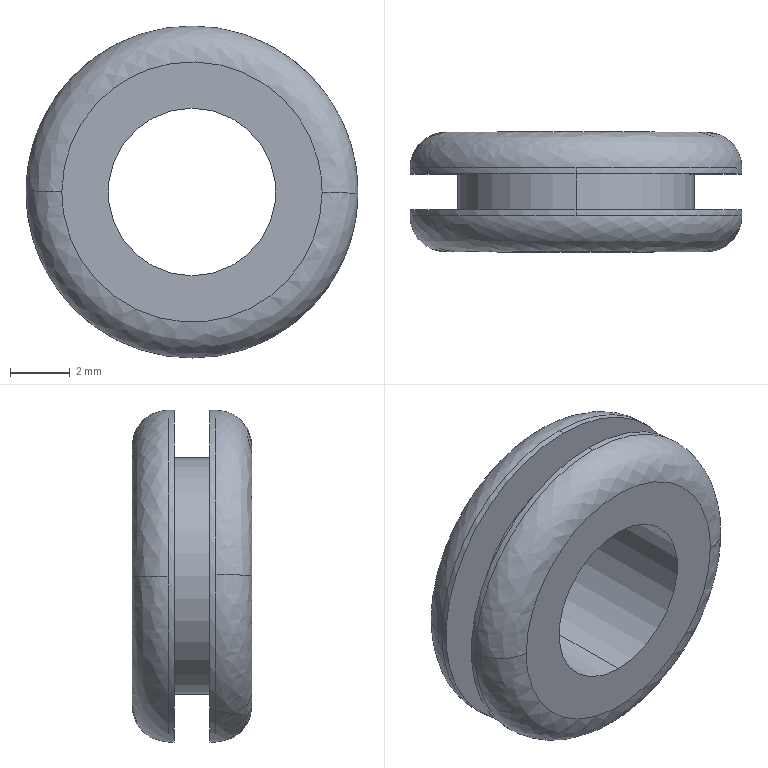Part | SolidWorks | features BaseBody 1 | 1 solid | 16 faces | box 11.1 x 4 x 11.1 mm | volume 210.744 mm3 | cylinder 8 | plane 4 | spline 4 | commonest cylinder face diameters 11.1 x4 5.6 x2 7.9 x2
STEP:
#1=CARTESIAN_POINT('',(0.,1.4,3.95));
#2=VERTEX_POINT('',#1);
#3=CARTESIAN_POINT('',(0.,1.4,-3.95));
#4=VERTEX_POINT('',#3);
#5=CARTESIAN_POINT('',(0.,1.4,0.));
#6=DIRECTION('',(0.,-1.,0.));
#7=DIRECTION('',(0.,0.,1.));
#8=AXIS2_PLACEMENT_3D('',#5,#6,#7);
#9=CIRCLE('',#8,3.95);
#10=EDGE_CURVE('',#2,#4,#9,.T.);
#11=ORIENTED_EDGE('',*,*,#10,.T.);
#12=CARTESIAN_POINT('',(0.,1.4,0.));
#13=DIRECTION('',(0.,-1.,0.));
#14=DIRECTION('',(0.,0.,1.));
#15=AXIS2_PLACEMENT_3D('',#12,#13,#14);
#16=CIRCLE('',#15,3.95);
#17=EDGE_CURVE('',#4,#2,#16,.T.);
#18=ORIENTED_EDGE('',*,*,#17,.T.);
#19=EDGE_LOOP('',(#11,#18));
#20=FACE_BOUND('',#19,.T.);
#21=CARTESIAN_POINT('',(0.,1.4,5.55));
#22=VERTEX_POINT('',#21);
#23=CARTESIAN_POINT('',(0.,1.4,-5.55));
#24=VERTEX_POINT('',#23);
#25=CARTESIAN_POINT('',(0.,1.4,0.));
#26=DIRECTION('',(0.,1.,0.));
#27=DIRECTION('',(0.,0.,1.));
#28=AXIS2_PLACEMENT_3D('',#25,#26,#27);
#29=CIRCLE('',#28,5.55);
#30=EDGE_CURVE('',#22,#24,#29,.T.);
#31=ORIENTED_EDGE('',*,*,#30,.T.);
#32=CARTESIAN_POINT('',(0.,1.4,0.));
#33=DIRECTION('',(0.,1.,0.));
#34=DIRECTION('',(0.,0.,1.));
#35=AXIS2_PLACEMENT_3D('',#32,#33,#34);
#36=CIRCLE('',#35,5.55);
#37=EDGE_CURVE('',#24,#22,#36,.T.);
#38=ORIENTED_EDGE('',*,*,#37,.T.);
#39=EDGE_LOOP('',(#31,#38));
#40=FACE_OUTER_BOUND('',#39,.T.);
#41=CARTESIAN_POINT('',(0.,1.4,0.));
#42=DIRECTION('',(0.,1.,0.));
#43=DIRECTION('',(1.,0.,0.));
#44=AXIS2_PLACEMENT_3D('',#41,#42,#43);
#45=PLANE('',#44);
#46=ADVANCED_FACE('',(#20,#40),#45,.T.);
#47=CARTESIAN_POINT('',(0.,2.6,-3.95));
#48=VERTEX_POINT('',#47);
#49=CARTESIAN_POINT('',(0.,1.4,-3.95));
#50=DIRECTION('',(0.,1.,0.));
#51=VECTOR('',#50,1000.);
#52=LINE('',#49,#51);
#53=EDGE_CURVE('',#4,#48,#52,.T.);
#54=ORIENTED_EDGE('',*,*,#53,.F.);
#55=ORIENTED_EDGE('',*,*,#10,.F.);
#56=CARTESIAN_POINT('',(0.,2.6,3.95));
#57=VERTEX_POINT('',#56);
#58=CARTESIAN_POINT('',(0.,1.4,3.95));
#59=DIRECTION('',(0.,1.,0.));
#60=VECTOR('',#59,1000.);
#61=LINE('',#58,#60);
#62=EDGE_CURVE('',#2,#57,#61,.T.);
#63=ORIENTED_EDGE('',*,*,#62,.T.);
#64=CARTESIAN_POINT('',(0.,2.6,0.));
#65=DIRECTION('',(0.,-1.,0.));
#66=DIRECTION('',(0.,0.,1.));
#67=AXIS2_PLACEMENT_3D('',#64,#65,#66);
#68=CIRCLE('',#67,3.95);
#69=EDGE_CURVE('',#57,#48,#68,.T.);
#70=ORIENTED_EDGE('',*,*,#69,.T.);
#71=EDGE_LOOP('',(#54,#55,#63,#70));
#72=FACE_OUTER_BOUND('',#71,.T.);
#73=CARTESIAN_POINT('',(0.,1.4,0.));
#74=DIRECTION('',(0.,1.,0.));
#75=DIRECTION('',(0.,0.,1.));
#76=AXIS2_PLACEMENT_3D('',#73,#74,#75);
#77=CYLINDRICAL_SURFACE('',#76,3.95);
#78=ADVANCED_FACE('',(#72),#77,.T.);
#79=CARTESIAN_POINT('',(0.,1.2,-5.55));
#80=VERTEX_POINT('',#79);
#81=CARTESIAN_POINT('',(0.,0.,-5.55));
#82=DIRECTION('',(0.,1.,0.));
#83=VECTOR('',#82,1000.);
#84=LINE('',#81,#83);
#85=EDGE_CURVE('',#80,#24,#84,.T.);
#86=ORIENTED_EDGE('',*,*,#85,.F.);
#87=CARTESIAN_POINT('',(-5.55,1.2,0.0354));
#88=VERTEX_POINT('',#87);
#89=CARTESIAN_POINT('',(0.,1.2,0.));
#90=DIRECTION('',(0.,1.,0.));
#91=DIRECTION('',(0.,0.,1.));
#92=AXIS2_PLACEMENT_3D('',#89,#90,#91);
#93=CIRCLE('',#92,5.55);
#94=EDGE_CURVE('',#80,#88,#93,.T.);
#95=ORIENTED_EDGE('',*,*,#94,.T.);
#96=CARTESIAN_POINT('',(0.,1.2,5.55));
#97=VERTEX_POINT('',#96);
#98=CARTESIAN_POINT('',(0.,1.2,0.));
#99=DIRECTION('',(0.,1.,0.));
#100=DIRECTION('',(0.,0.,1.));
#101=AXIS2_PLACEMENT_3D('',#98,#99,#100);
#102=CIRCLE('',#101,5.55);
#103=EDGE_CURVE('',#88,#97,#102,.T.);
#104=ORIENTED_EDGE('',*,*,#103,.T.);
#105=CARTESIAN_POINT('',(0.,0.,5.55));
#106=DIRECTION('',(0.,1.,0.));
#107=VECTOR('',#106,1000.);
#108=LINE('',#105,#107);
#109=EDGE_CURVE('',#97,#22,#108,.T.);
#110=ORIENTED_EDGE('',*,*,#109,.T.);
#111=ORIENTED_EDGE('',*,*,#37,.F.);
#112=EDGE_LOOP('',(#86,#95,#104,#110,#111));
#113=FACE_OUTER_BOUND('',#112,.T.);
#114=CARTESIAN_POINT('',(0.,0.,0.));
#115=DIRECTION('',(0.,1.,0.));
#116=DIRECTION('',(0.,0.,1.));
#117=AXIS2_PLACEMENT_3D('',#114,#115,#116);
#118=CYLINDRICAL_SURFACE('',#117,5.55);
#119=ADVANCED_FACE('',(#113),#118,.T.);
#120=ORIENTED_EDGE('',*,*,#69,.F.);
#121=CARTESIAN_POINT('',(0.,2.6,0.));
#122=DIRECTION('',(0.,-1.,0.));
#123=DIRECTION('',(0.,0.,1.));
#124=AXIS2_PLACEMENT_3D('',#121,#122,#123);
#125=CIRCLE('',#124,3.95);
#126=EDGE_CURVE('',#48,#57,#125,.T.);
#127=ORIENTED_EDGE('',*,*,#126,.F.);
#128=EDGE_LOOP('',(#120,#127));
#129=FACE_BOUND('',#128,.T.);
#130=CARTESIAN_POINT('',(0.,2.6,5.55));
#131=VERTEX_POINT('',#130);
#132=CARTESIAN_POINT('',(0.,2.6,-5.55));
#133=VERTEX_POINT('',#132);
#134=CARTESIAN_POINT('',(0.,2.6,0.));
#135=DIRECTION('',(0.,1.,0.));
#136=DIRECTION('',(0.,0.,1.));
#137=AXIS2_PLACEMENT_3D('',#134,#135,#136);
#138=CIRCLE('',#137,5.55);
#139=EDGE_CURVE('',#131,#133,#138,.T.);
#140=ORIENTED_EDGE('',*,*,#139,.F.);
#141=CARTESIAN_POINT('',(0.,2.6,0.));
#142=DIRECTION('',(0.,1.,0.));
#143=DIRECTION('',(0.,0.,1.));
#144=AXIS2_PLACEMENT_3D('',#141,#142,#143);
#145=CIRCLE('',#144,5.55);
#146=EDGE_CURVE('',#133,#131,#145,.T.);
#147=ORIENTED_EDGE('',*,*,#146,.F.);
#148=EDGE_LOOP('',(#140,#147));
#149=FACE_OUTER_BOUND('',#148,.T.);
#150=CARTESIAN_POINT('',(0.,2.6,0.));
#151=DIRECTION('',(0.,1.,0.));
#152=DIRECTION('',(1.,0.,0.));
#153=AXIS2_PLACEMENT_3D('',#150,#151,#152);
#154=PLANE('',#153);
#155=ADVANCED_FACE('',(#129,#149),#154,.F.);
#156=CARTESIAN_POINT('',(5.55,1.2,-0.0354));
#157=VERTEX_POINT('',#156);
#158=CARTESIAN_POINT('',(4.35,0.,-0.02774));
#159=VERTEX_POINT('',#158);
#160=CARTESIAN_POINT('',(4.35,1.2,-0.02774));
#161=DIRECTION('',(-0.006378,0.,-1.));
#162=DIRECTION('',(1.,0.,-0.006378));
#163=AXIS2_PLACEMENT_3D('',#160,#161,#162);
#164=CIRCLE('',#163,1.2);
#165=EDGE_CURVE('',#157,#159,#164,.T.);
#166=ORIENTED_EDGE('',*,*,#165,.F.);
#167=CARTESIAN_POINT('',(0.,1.2,0.));
#168=DIRECTION('',(0.,1.,0.));
#169=DIRECTION('',(0.,0.,1.));
#170=AXIS2_PLACEMENT_3D('',#167,#168,#169);
#171=CIRCLE('',#170,5.55);
#172=EDGE_CURVE('',#97,#157,#171,.T.);
#173=ORIENTED_EDGE('',*,*,#172,.F.);
#174=ORIENTED_EDGE('',*,*,#103,.F.);
#175=CARTESIAN_POINT('',(-4.35,0.,0.02774));
#176=VERTEX_POINT('',#175);
#177=CARTESIAN_POINT('',(-4.35,1.2,0.02774));
#178=DIRECTION('',(0.006378,0.,1.));
#179=DIRECTION('',(-1.,0.,0.006378));
#180=AXIS2_PLACEMENT_3D('',#177,#178,#179);
#181=CIRCLE('',#180,1.2);
#182=EDGE_CURVE('',#88,#176,#181,.T.);
#183=ORIENTED_EDGE('',*,*,#182,.T.);
#184=CARTESIAN_POINT('',(4.35,0.,0.));
#185=VERTEX_POINT('',#184);
#186=CARTESIAN_POINT('',(-4.35,0.,0.02774));
#187=CARTESIAN_POINT('',(-4.347,0.,0.4058));
#188=CARTESIAN_POINT('',(-4.295,0.00000001,0.833));
#189=CARTESIAN_POINT('',(-4.016,0.000000026,1.737));
#190=CARTESIAN_POINT('',(-3.787,0.000000032,2.214));
#191=CARTESIAN_POINT('',(-3.091,0.000000032,3.113));
#192=CARTESIAN_POINT('',(-2.622,0.000000026,3.533));
#193=CARTESIAN_POINT('',(-1.743,0.000000014,3.999));
#194=CARTESIAN_POINT('',(-1.421,0.00000001,4.126));
#195=CARTESIAN_POINT('',(-0.9047,0.000000004,4.258));
#196=CARTESIAN_POINT('',(-0.7269,0.000000003,4.293));
#197=CARTESIAN_POINT('',(-0.4535,0.000000001,4.327));
#198=CARTESIAN_POINT('',(-0.3613,0.000000001,4.336));
#199=CARTESIAN_POINT('',(-0.2216,0.,4.345));
#200=CARTESIAN_POINT('',(-0.1514,0.,4.348));
#201=CARTESIAN_POINT('',(-0.06892,0.,4.35));
#202=CARTESIAN_POINT('',(-0.02757,0.,4.35));
#203=CARTESIAN_POINT('',(-0.009816,0.,4.35));
#204=CARTESIAN_POINT('',(0.002023,0.,4.35));
#205=CARTESIAN_POINT('',(0.009432,0.,4.35));
#206=CARTESIAN_POINT('',(0.5821,0.,4.348));
#207=CARTESIAN_POINT('',(1.15,0.000000006,4.234));
#208=CARTESIAN_POINT('',(2.199,0.000000015,3.796));
#209=CARTESIAN_POINT('',(2.68,0.000000018,3.474));
#210=CARTESIAN_POINT('',(3.482,0.000000018,2.669));
#211=CARTESIAN_POINT('',(3.803,0.000000015,2.187));
#212=CARTESIAN_POINT('',(4.237,0.000000006,1.136));
#213=CARTESIAN_POINT('',(4.35,0.,0.5683));
#214=CARTESIAN_POINT('',(4.35,0.,0.));
#215=B_SPLINE_CURVE_WITH_KNOTS('',3,(#186,#187,#188,#189,#190,#191,#192,#193,#194,#195,#196,#197,#198,#199,#200,#201,#202,#203,#204,#205,#206,#207,#208,#209,#210,#211,#212,#213,#214),.UNSPECIFIED.,.F.,.F.,(4,2,2,2,2,2,2,1,1,1,2,2,2,2,2,4),(0.,0.125,0.25,0.375,0.4375,0.4688,0.4844,0.4922,0.4961,0.498,0.499,0.5,0.625,0.75,0.875,1.),.UNSPECIFIED.);
#216=EDGE_CURVE('',#176,#185,#215,.T.);
#217=ORIENTED_EDGE('',*,*,#216,.T.);
#218=CARTESIAN_POINT('',(4.35,0.,-0.02774));
#219=DIRECTION('',(-0.003189,0.,-1.));
#220=VECTOR('',#219,1000.);
#221=LINE('',#218,#220);
#222=EDGE_CURVE('',#185,#159,#221,.T.);
#223=ORIENTED_EDGE('',*,*,#222,.T.);
#224=EDGE_LOOP('',(#166,#173,#174,#183,#217,#223));
#225=FACE_OUTER_BOUND('',#224,.T.);
#226=CARTESIAN_POINT('',(-5.55,1.2,0.0354));
#227=CARTESIAN_POINT('',(-5.479,1.2,11.135));
#228=CARTESIAN_POINT('',(5.621,1.2,11.064));
#229=CARTESIAN_POINT('',(5.55,1.2,-0.0354));
#230=CARTESIAN_POINT('',(-5.55,0.4917,0.0354));
#231=CARTESIAN_POINT('',(-5.479,0.4917,11.135));
#232=CARTESIAN_POINT('',(5.621,0.4917,11.064));
#233=CARTESIAN_POINT('',(5.55,0.4917,-0.0354));
#234=CARTESIAN_POINT('',(-5.047,-0.006784,0.03219));
#235=CARTESIAN_POINT('',(-4.982,-0.006784,10.125));
#236=CARTESIAN_POINT('',(5.111,-0.006784,10.061));
#237=CARTESIAN_POINT('',(5.047,-0.006784,-0.03219));
#238=CARTESIAN_POINT('',(-4.338,0.00005595,0.02767));
#239=CARTESIAN_POINT('',(-4.283,0.00005595,8.704));
#240=CARTESIAN_POINT('',(4.394,0.00005595,8.649));
#241=CARTESIAN_POINT('',(4.338,0.00005595,-0.02767));
#242=(BOUNDED_SURFACE()B_SPLINE_SURFACE(3,3,((#226,#227,#228,#229),(#230,#231,#232,#233),(#234,#235,#236,#237),(#238,#239,#240,#241)),.UNSPECIFIED.,.F.,.F.,.T.)B_SPLINE_SURFACE_WITH_KNOTS((4,4),(4,4),(0.,1.),(0.,1.),.UNSPECIFIED.)GEOMETRIC_REPRESENTATION_ITEM()RATIONAL_B_SPLINE_SURFACE(((1.,0.3333,0.3333,1.),(0.8025,0.2675,0.2675,0.8025),(0.8025,0.2675,0.2675,0.8025),(1.,0.3333,0.3333,1.)))REPRESENTATION_ITEM('')SURFACE());
#243=ADVANCED_FACE('',(#225),#242,.T.);
#244=CARTESIAN_POINT('',(0.,2.8,-5.55));
#245=VERTEX_POINT('',#244);
#246=CARTESIAN_POINT('',(0.,0.,-5.55));
#247=DIRECTION('',(0.,1.,0.));
#248=VECTOR('',#247,1000.);
#249=LINE('',#246,#248);
#250=EDGE_CURVE('',#133,#245,#249,.T.);
#251=ORIENTED_EDGE('',*,*,#250,.F.);
#252=ORIENTED_EDGE('',*,*,#146,.T.);
#253=CARTESIAN_POINT('',(0.,2.8,5.55));
#254=VERTEX_POINT('',#253);
#255=CARTESIAN_POINT('',(0.,0.,5.55));
#256=DIRECTION('',(0.,1.,0.));
#257=VECTOR('',#256,1000.);
#258=LINE('',#255,#257);
#259=EDGE_CURVE('',#131,#254,#258,.T.);
#260=ORIENTED_EDGE('',*,*,#259,.T.);
#261=CARTESIAN_POINT('',(-5.55,2.8,-0.02492));
#262=VERTEX_POINT('',#261);
#263=CARTESIAN_POINT('',(0.,2.8,0.));
#264=DIRECTION('',(0.,-1.,0.));
#265=DIRECTION('',(0.,0.,1.));
#266=AXIS2_PLACEMENT_3D('',#263,#264,#265);
#267=CIRCLE('',#266,5.55);
#268=EDGE_CURVE('',#254,#262,#267,.T.);
#269=ORIENTED_EDGE('',*,*,#268,.T.);
#270=CARTESIAN_POINT('',(0.,2.8,0.));
#271=DIRECTION('',(0.,-1.,0.));
#272=DIRECTION('',(0.,0.,1.));
#273=AXIS2_PLACEMENT_3D('',#270,#271,#272);
#274=CIRCLE('',#273,5.55);
#275=EDGE_CURVE('',#262,#245,#274,.T.);
#276=ORIENTED_EDGE('',*,*,#275,.T.);
#277=EDGE_LOOP('',(#251,#252,#260,#269,#276));
#278=FACE_OUTER_BOUND('',#277,.T.);
#279=CARTESIAN_POINT('',(0.,0.,0.));
#280=DIRECTION('',(0.,1.,0.));
#281=DIRECTION('',(0.,0.,1.));
#282=AXIS2_PLACEMENT_3D('',#279,#280,#281);
#283=CYLINDRICAL_SURFACE('',#282,5.55);
#284=ADVANCED_FACE('',(#278),#283,.T.);
#285=CARTESIAN_POINT('',(0.,0.,2.8));
#286=VERTEX_POINT('',#285);
#287=CARTESIAN_POINT('',(0.,0.,-2.8));
#288=VERTEX_POINT('',#287);
#289=CARTESIAN_POINT('',(0.,0.,0.));
#290=DIRECTION('',(0.,-1.,0.));
#291=DIRECTION('',(0.,0.,1.));
#292=AXIS2_PLACEMENT_3D('',#289,#290,#291);
#293=CIRCLE('',#292,2.8);
#294=EDGE_CURVE('',#286,#288,#293,.T.);
#295=ORIENTED_EDGE('',*,*,#294,.F.);
#296=CARTESIAN_POINT('',(0.,0.,0.));
#297=DIRECTION('',(0.,-1.,0.));
#298=DIRECTION('',(0.,0.,1.));
#299=AXIS2_PLACEMENT_3D('',#296,#297,#298);
#300=CIRCLE('',#299,2.8);
#301=EDGE_CURVE('',#288,#286,#300,.T.);
#302=ORIENTED_EDGE('',*,*,#301,.F.);
#303=EDGE_LOOP('',(#295,#302));
#304=FACE_BOUND('',#303,.T.);
#305=ORIENTED_EDGE('',*,*,#222,.F.);
#306=ORIENTED_EDGE('',*,*,#216,.F.);
#307=CARTESIAN_POINT('',(-4.35,0.,0.));
#308=VERTEX_POINT('',#307);
#309=CARTESIAN_POINT('',(-4.35,0.,0.02774));
#310=DIRECTION('',(0.003189,0.,1.));
#311=VECTOR('',#310,1000.);
#312=LINE('',#309,#311);
#313=EDGE_CURVE('',#308,#176,#312,.T.);
#314=ORIENTED_EDGE('',*,*,#313,.F.);
#315=CARTESIAN_POINT('',(4.35,0.,-0.02774));
#316=CARTESIAN_POINT('',(4.295,0.,-8.672));
#317=CARTESIAN_POINT('',(-4.35,0.,-8.645));
#318=CARTESIAN_POINT('',(-4.35,0.,0.));
#319=(BOUNDED_CURVE()B_SPLINE_CURVE(3,(#315,#316,#317,#318),.UNSPECIFIED.,.F.,.T.)B_SPLINE_CURVE_WITH_KNOTS((4,4),(0.,1.),.UNSPECIFIED.)CURVE()GEOMETRIC_REPRESENTATION_ITEM()RATIONAL_B_SPLINE_CURVE((1.,0.3355,0.3355,1.))REPRESENTATION_ITEM(''));
#320=EDGE_CURVE('',#159,#308,#319,.T.);
#321=ORIENTED_EDGE('',*,*,#320,.F.);
#322=EDGE_LOOP('',(#305,#306,#314,#321));
#323=FACE_OUTER_BOUND('',#322,.T.);
#324=CARTESIAN_POINT('',(0.,0.,0.));
#325=DIRECTION('',(0.,1.,0.));
#326=DIRECTION('',(1.,0.,0.));
#327=AXIS2_PLACEMENT_3D('',#324,#325,#326);
#328=PLANE('',#327);
#329=ADVANCED_FACE('',(#304,#323),#328,.F.);
#330=CARTESIAN_POINT('',(4.35,4.,0.01953));
#331=VERTEX_POINT('',#330);
#332=CARTESIAN_POINT('',(5.55,2.8,0.02492));
#333=VERTEX_POINT('',#332);
#334=CARTESIAN_POINT('',(4.35,2.8,0.01953));
#335=DIRECTION('',(0.00449,0.,-1.));
#336=DIRECTION('',(1.,0.,0.00449));
#337=AXIS2_PLACEMENT_3D('',#334,#335,#336);
#338=CIRCLE('',#337,1.2);
#339=EDGE_CURVE('',#331,#333,#338,.T.);
#340=ORIENTED_EDGE('',*,*,#339,.F.);
#341=CARTESIAN_POINT('',(-4.35,4.,0.));
#342=VERTEX_POINT('',#341);
#343=CARTESIAN_POINT('',(4.35,4.,0.01953));
#344=CARTESIAN_POINT('',(4.311,4.,8.681));
#345=CARTESIAN_POINT('',(-4.35,4.,8.661));
#346=CARTESIAN_POINT('',(-4.35,4.,0.));
#347=(BOUNDED_CURVE()B_SPLINE_CURVE(3,(#343,#344,#345,#346),.UNSPECIFIED.,.F.,.F.)B_SPLINE_CURVE_WITH_KNOTS((4,4),(0.,1.),.UNSPECIFIED.)CURVE()GEOMETRIC_REPRESENTATION_ITEM()RATIONAL_B_SPLINE_CURVE((1.,0.3348,0.3348,1.))REPRESENTATION_ITEM(''));
#348=EDGE_CURVE('',#331,#342,#347,.T.);
#349=ORIENTED_EDGE('',*,*,#348,.T.);
#350=CARTESIAN_POINT('',(-4.35,4.,-0.01953));
#351=VERTEX_POINT('',#350);
#352=CARTESIAN_POINT('',(-4.35,4.,-0.01953));
#353=DIRECTION('',(0.002245,0.,-1.));
#354=VECTOR('',#353,1000.);
#355=LINE('',#352,#354);
#356=EDGE_CURVE('',#342,#351,#355,.T.);
#357=ORIENTED_EDGE('',*,*,#356,.T.);
#358=CARTESIAN_POINT('',(-4.35,2.8,-0.01953));
#359=DIRECTION('',(-0.00449,0.,1.));
#360=DIRECTION('',(-1.,0.,-0.00449));
#361=AXIS2_PLACEMENT_3D('',#358,#359,#360);
#362=CIRCLE('',#361,1.2);
#363=EDGE_CURVE('',#351,#262,#362,.T.);
#364=ORIENTED_EDGE('',*,*,#363,.T.);
#365=ORIENTED_EDGE('',*,*,#268,.F.);
#366=CARTESIAN_POINT('',(0.,2.8,0.));
#367=DIRECTION('',(0.,-1.,0.));
#368=DIRECTION('',(0.,0.,1.));
#369=AXIS2_PLACEMENT_3D('',#366,#367,#368);
#370=CIRCLE('',#369,5.55);
#371=EDGE_CURVE('',#333,#254,#370,.T.);
#372=ORIENTED_EDGE('',*,*,#371,.F.);
#373=EDGE_LOOP('',(#340,#349,#357,#364,#365,#372));
#374=FACE_OUTER_BOUND('',#373,.T.);
#375=CARTESIAN_POINT('',(-4.339,4.,-0.01948));
#376=CARTESIAN_POINT('',(-4.35,4.,2.541));
#377=CARTESIAN_POINT('',(-2.539,4.,4.351));
#378=CARTESIAN_POINT('',(0.02141,4.,4.339));
#379=CARTESIAN_POINT('',(2.582,4.,4.326));
#380=CARTESIAN_POINT('',(4.375,4.,2.498));
#381=CARTESIAN_POINT('',(4.338,4.,-0.0623));
#382=CARTESIAN_POINT('',(-5.047,4.007,-0.02266));
#383=CARTESIAN_POINT('',(-5.06,4.007,2.956));
#384=CARTESIAN_POINT('',(-2.954,4.007,5.061));
#385=CARTESIAN_POINT('',(0.02491,4.007,5.047));
#386=CARTESIAN_POINT('',(3.003,4.007,5.032));
#387=CARTESIAN_POINT('',(5.089,4.007,2.906));
#388=CARTESIAN_POINT('',(5.046,4.007,-0.07247));
#389=CARTESIAN_POINT('',(-5.55,3.508,-0.02492));
#390=CARTESIAN_POINT('',(-5.565,3.508,3.251));
#391=CARTESIAN_POINT('',(-3.248,3.508,5.566));
#392=CARTESIAN_POINT('',(0.02739,3.508,5.55));
#393=CARTESIAN_POINT('',(3.303,3.508,5.534));
#394=CARTESIAN_POINT('',(5.596,3.508,3.195));
#395=CARTESIAN_POINT('',(5.549,3.508,-0.07969));
#396=CARTESIAN_POINT('',(-5.55,2.8,-0.02492));
#397=CARTESIAN_POINT('',(-5.565,2.8,3.251));
#398=CARTESIAN_POINT('',(-3.248,2.8,5.566));
#399=CARTESIAN_POINT('',(0.02739,2.8,5.55));
#400=CARTESIAN_POINT('',(3.303,2.8,5.534));
#401=CARTESIAN_POINT('',(5.596,2.8,3.195));
#402=CARTESIAN_POINT('',(5.549,2.8,-0.07969));
#403=(BOUNDED_SURFACE()B_SPLINE_SURFACE(3,3,((#375,#376,#377,#378,#379,#380,#381),(#382,#383,#384,#385,#386,#387,#388),(#389,#390,#391,#392,#393,#394,#395),(#396,#397,#398,#399,#400,#401,#402)),.UNSPECIFIED.,.F.,.F.,.T.)B_SPLINE_SURFACE_WITH_KNOTS((4,4),(4,3,4),(0.,1.),(0.,0.5,1.),.UNSPECIFIED.)GEOMETRIC_REPRESENTATION_ITEM()RATIONAL_B_SPLINE_SURFACE(((1.,0.8025,0.8025,1.,0.8025,0.8025,1.),(0.8025,0.644,0.644,0.8025,0.644,0.644,0.8025),(0.8025,0.644,0.644,0.8025,0.644,0.644,0.8025),(1.,0.8025,0.8025,1.,0.8025,0.8025,1.)))REPRESENTATION_ITEM('')SURFACE());
#404=ADVANCED_FACE('',(#374),#403,.T.);
#405=CARTESIAN_POINT('',(0.,4.,-2.8));
#406=VERTEX_POINT('',#405);
#407=CARTESIAN_POINT('',(0.,4.,-2.8));
#408=DIRECTION('',(0.,1.,0.));
#409=VECTOR('',#408,1000.);
#410=LINE('',#407,#409);
#411=EDGE_CURVE('',#288,#406,#410,.T.);
#412=ORIENTED_EDGE('',*,*,#411,.F.);
#413=ORIENTED_EDGE('',*,*,#301,.T.);
#414=CARTESIAN_POINT('',(0.,4.,2.8));
#415=VERTEX_POINT('',#414);
#416=CARTESIAN_POINT('',(0.,4.,2.8));
#417=DIRECTION('',(0.,1.,0.));
#418=VECTOR('',#417,1000.);
#419=LINE('',#416,#418);
#420=EDGE_CURVE('',#286,#415,#419,.T.);
#421=ORIENTED_EDGE('',*,*,#420,.T.);
#422=CARTESIAN_POINT('',(0.,4.,0.));
#423=DIRECTION('',(0.,-1.,0.));
#424=DIRECTION('',(0.,0.,1.));
#425=AXIS2_PLACEMENT_3D('',#422,#423,#424);
#426=CIRCLE('',#425,2.8);
#427=EDGE_CURVE('',#406,#415,#426,.T.);
#428=ORIENTED_EDGE('',*,*,#427,.F.);
#429=EDGE_LOOP('',(#412,#413,#421,#428));
#430=FACE_OUTER_BOUND('',#429,.T.);
#431=CARTESIAN_POINT('',(0.,4.,0.));
#432=DIRECTION('',(0.,1.,0.));
#433=DIRECTION('',(0.,0.,1.));
#434=AXIS2_PLACEMENT_3D('',#431,#432,#433);
#435=CYLINDRICAL_SURFACE('',#434,2.8);
#436=ADVANCED_FACE('',(#430),#435,.F.);
#437=CARTESIAN_POINT('',(0.,4.,0.));
#438=DIRECTION('',(0.,-1.,0.));
#439=DIRECTION('',(0.,0.,1.));
#440=AXIS2_PLACEMENT_3D('',#437,#438,#439);
#441=CIRCLE('',#440,2.8);
#442=EDGE_CURVE('',#415,#406,#441,.T.);
#443=ORIENTED_EDGE('',*,*,#442,.T.);
#444=ORIENTED_EDGE('',*,*,#427,.T.);
#445=EDGE_LOOP('',(#443,#444));
#446=FACE_BOUND('',#445,.T.);
#447=ORIENTED_EDGE('',*,*,#348,.F.);
#448=CARTESIAN_POINT('',(4.35,4.,0.));
#449=VERTEX_POINT('',#448);
#450=CARTESIAN_POINT('',(4.35,4.,0.01953));
#451=DIRECTION('',(-0.002245,0.,1.));
#452=VECTOR('',#451,1000.);
#453=LINE('',#450,#452);
#454=EDGE_CURVE('',#449,#331,#453,.T.);
#455=ORIENTED_EDGE('',*,*,#454,.F.);
#456=CARTESIAN_POINT('',(-4.35,4.,-0.01953));
#457=CARTESIAN_POINT('',(-4.347,4.,-0.5881));
#458=CARTESIAN_POINT('',(-4.232,4.,-1.156));
#459=CARTESIAN_POINT('',(-3.792,4.,-2.205));
#460=CARTESIAN_POINT('',(-3.469,4.,-2.685));
#461=CARTESIAN_POINT('',(-2.662,4.,-3.487));
#462=CARTESIAN_POINT('',(-2.179,4.,-3.807));
#463=CARTESIAN_POINT('',(-1.127,4.,-4.239));
#464=CARTESIAN_POINT('',(-0.5588,4.,-4.351));
#465=CARTESIAN_POINT('',(0.5784,4.,-4.349));
#466=CARTESIAN_POINT('',(1.147,4.,-4.235));
#467=CARTESIAN_POINT('',(2.197,4.,-3.798));
#468=CARTESIAN_POINT('',(2.678,4.,-3.475));
#469=CARTESIAN_POINT('',(3.481,4.,-2.67));
#470=CARTESIAN_POINT('',(3.803,4.,-2.188));
#471=CARTESIAN_POINT('',(4.237,4.,-1.137));
#472=CARTESIAN_POINT('',(4.35,4.,-0.5686));
#473=CARTESIAN_POINT('',(4.35,4.,0.));
#474=B_SPLINE_CURVE_WITH_KNOTS('',3,(#456,#457,#458,#459,#460,#461,#462,#463,#464,#465,#466,#467,#468,#469,#470,#471,#472,#473),.UNSPECIFIED.,.F.,.F.,(4,2,2,2,2,2,2,2,4),(0.,0.125,0.25,0.375,0.5,0.625,0.75,0.875,1.),.UNSPECIFIED.);
#475=EDGE_CURVE('',#351,#449,#474,.T.);
#476=ORIENTED_EDGE('',*,*,#475,.F.);
#477=ORIENTED_EDGE('',*,*,#356,.F.);
#478=EDGE_LOOP('',(#447,#455,#476,#477));
#479=FACE_OUTER_BOUND('',#478,.T.);
#480=CARTESIAN_POINT('',(0.,4.,0.));
#481=DIRECTION('',(0.,1.,0.));
#482=DIRECTION('',(1.,0.,0.));
#483=AXIS2_PLACEMENT_3D('',#480,#481,#482);
#484=PLANE('',#483);
#485=ADVANCED_FACE('',(#446,#479),#484,.T.);
#486=ORIENTED_EDGE('',*,*,#294,.T.);
#487=ORIENTED_EDGE('',*,*,#411,.T.);
#488=ORIENTED_EDGE('',*,*,#442,.F.);
#489=ORIENTED_EDGE('',*,*,#420,.F.);
#490=EDGE_LOOP('',(#486,#487,#488,#489));
#491=FACE_OUTER_BOUND('',#490,.T.);
#492=CARTESIAN_POINT('',(0.,4.,0.));
#493=DIRECTION('',(0.,1.,0.));
#494=DIRECTION('',(0.,0.,1.));
#495=AXIS2_PLACEMENT_3D('',#492,#493,#494);
#496=CYLINDRICAL_SURFACE('',#495,2.8);
#497=ADVANCED_FACE('',(#491),#496,.F.);
#498=ORIENTED_EDGE('',*,*,#139,.T.);
#499=ORIENTED_EDGE('',*,*,#250,.T.);
#500=CARTESIAN_POINT('',(0.,2.8,0.));
#501=DIRECTION('',(0.,-1.,0.));
#502=DIRECTION('',(0.,0.,1.));
#503=AXIS2_PLACEMENT_3D('',#500,#501,#502);
#504=CIRCLE('',#503,5.55);
#505=EDGE_CURVE('',#245,#333,#504,.T.);
#506=ORIENTED_EDGE('',*,*,#505,.T.);
#507=ORIENTED_EDGE('',*,*,#371,.T.);
#508=ORIENTED_EDGE('',*,*,#259,.F.);
#509=EDGE_LOOP('',(#498,#499,#506,#507,#508));
#510=FACE_OUTER_BOUND('',#509,.T.);
#511=CARTESIAN_POINT('',(0.,0.,0.));
#512=DIRECTION('',(0.,1.,0.));
#513=DIRECTION('',(0.,0.,1.));
#514=AXIS2_PLACEMENT_3D('',#511,#512,#513);
#515=CYLINDRICAL_SURFACE('',#514,5.55);
#516=ADVANCED_FACE('',(#510),#515,.T.);
#517=ORIENTED_EDGE('',*,*,#172,.T.);
#518=CARTESIAN_POINT('',(0.,1.2,0.));
#519=DIRECTION('',(0.,1.,0.));
#520=DIRECTION('',(0.,0.,1.));
#521=AXIS2_PLACEMENT_3D('',#518,#519,#520);
#522=CIRCLE('',#521,5.55);
#523=EDGE_CURVE('',#157,#80,#522,.T.);
#524=ORIENTED_EDGE('',*,*,#523,.T.);
#525=ORIENTED_EDGE('',*,*,#85,.T.);
#526=ORIENTED_EDGE('',*,*,#30,.F.);
#527=ORIENTED_EDGE('',*,*,#109,.F.);
#528=EDGE_LOOP('',(#517,#524,#525,#526,#527));
#529=FACE_OUTER_BOUND('',#528,.T.);
#530=CARTESIAN_POINT('',(0.,0.,0.));
#531=DIRECTION('',(0.,1.,0.));
#532=DIRECTION('',(0.,0.,1.));
#533=AXIS2_PLACEMENT_3D('',#530,#531,#532);
#534=CYLINDRICAL_SURFACE('',#533,5.55);
#535=ADVANCED_FACE('',(#529),#534,.T.);
#536=ORIENTED_EDGE('',*,*,#17,.F.);
#537=ORIENTED_EDGE('',*,*,#53,.T.);
#538=ORIENTED_EDGE('',*,*,#126,.T.);
#539=ORIENTED_EDGE('',*,*,#62,.F.);
#540=EDGE_LOOP('',(#536,#537,#538,#539));
#541=FACE_OUTER_BOUND('',#540,.T.);
#542=CARTESIAN_POINT('',(0.,1.4,0.));
#543=DIRECTION('',(0.,1.,0.));
#544=DIRECTION('',(0.,0.,1.));
#545=AXIS2_PLACEMENT_3D('',#542,#543,#544);
#546=CYLINDRICAL_SURFACE('',#545,3.95);
#547=ADVANCED_FACE('',(#541),#546,.T.);
#548=ORIENTED_EDGE('',*,*,#454,.T.);
#549=ORIENTED_EDGE('',*,*,#339,.T.);
#550=ORIENTED_EDGE('',*,*,#505,.F.);
#551=ORIENTED_EDGE('',*,*,#275,.F.);
#552=ORIENTED_EDGE('',*,*,#363,.F.);
#553=ORIENTED_EDGE('',*,*,#475,.T.);
#554=EDGE_LOOP('',(#548,#549,#550,#551,#552,#553));
#555=FACE_OUTER_BOUND('',#554,.T.);
#556=CARTESIAN_POINT('',(4.338,4.,0.01948));
#557=CARTESIAN_POINT('',(4.377,4.,-8.657));
#558=CARTESIAN_POINT('',(-4.299,4.,-8.696));
#559=CARTESIAN_POINT('',(-4.338,4.,-0.01948));
#560=CARTESIAN_POINT('',(5.047,4.007,0.02266));
#561=CARTESIAN_POINT('',(5.092,4.007,-10.071));
#562=CARTESIAN_POINT('',(-5.001,4.007,-10.116));
#563=CARTESIAN_POINT('',(-5.047,4.007,-0.02266));
#564=CARTESIAN_POINT('',(5.55,3.508,0.02492));
#565=CARTESIAN_POINT('',(5.6,3.508,-11.075));
#566=CARTESIAN_POINT('',(-5.5,3.508,-11.125));
#567=CARTESIAN_POINT('',(-5.55,3.508,-0.02492));
#568=CARTESIAN_POINT('',(5.55,2.8,0.02492));
#569=CARTESIAN_POINT('',(5.6,2.8,-11.075));
#570=CARTESIAN_POINT('',(-5.5,2.8,-11.125));
#571=CARTESIAN_POINT('',(-5.55,2.8,-0.02492));
#572=(BOUNDED_SURFACE()B_SPLINE_SURFACE(3,3,((#556,#557,#558,#559),(#560,#561,#562,#563),(#564,#565,#566,#567),(#568,#569,#570,#571)),.UNSPECIFIED.,.F.,.F.,.T.)B_SPLINE_SURFACE_WITH_KNOTS((4,4),(4,4),(0.,1.),(0.,1.),.UNSPECIFIED.)GEOMETRIC_REPRESENTATION_ITEM()RATIONAL_B_SPLINE_SURFACE(((1.,0.3333,0.3333,1.),(0.8024,0.2675,0.2675,0.8024),(0.8024,0.2675,0.2675,0.8024),(1.,0.3333,0.3333,1.)))REPRESENTATION_ITEM('')SURFACE());
#573=ADVANCED_FACE('',(#555),#572,.T.);
#574=ORIENTED_EDGE('',*,*,#523,.F.);
#575=ORIENTED_EDGE('',*,*,#165,.T.);
#576=ORIENTED_EDGE('',*,*,#320,.T.);
#577=ORIENTED_EDGE('',*,*,#313,.T.);
#578=ORIENTED_EDGE('',*,*,#182,.F.);
#579=ORIENTED_EDGE('',*,*,#94,.F.);
#580=EDGE_LOOP('',(#574,#575,#576,#577,#578,#579));
#581=FACE_OUTER_BOUND('',#580,.T.);
#582=CARTESIAN_POINT('',(5.55,1.2,0.06922));
#583=CARTESIAN_POINT('',(5.59,1.2,-3.206));
#584=CARTESIAN_POINT('',(3.292,1.2,-5.54));
#585=CARTESIAN_POINT('',(0.01691,1.2,-5.55));
#586=CARTESIAN_POINT('',(-3.259,1.2,-5.56));
#587=CARTESIAN_POINT('',(-5.571,1.2,-3.24));
#588=CARTESIAN_POINT('',(-5.55,1.2,0.0354));
#589=CARTESIAN_POINT('',(5.55,0.4918,0.06922));
#590=CARTESIAN_POINT('',(5.59,0.4918,-3.206));
#591=CARTESIAN_POINT('',(3.292,0.4918,-5.54));
#592=CARTESIAN_POINT('',(0.01691,0.4918,-5.55));
#593=CARTESIAN_POINT('',(-3.259,0.4918,-5.56));
#594=CARTESIAN_POINT('',(-5.571,0.4918,-3.24));
#595=CARTESIAN_POINT('',(-5.55,0.4918,0.0354));
#596=CARTESIAN_POINT('',(5.046,-0.006639,0.06294));
#597=CARTESIAN_POINT('',(5.084,-0.006639,-2.915));
#598=CARTESIAN_POINT('',(2.994,-0.006639,-5.038));
#599=CARTESIAN_POINT('',(0.01538,-0.006639,-5.047));
#600=CARTESIAN_POINT('',(-2.963,-0.006639,-5.056));
#601=CARTESIAN_POINT('',(-5.066,-0.006639,-2.946));
#602=CARTESIAN_POINT('',(-5.047,-0.006639,0.03219));
#603=CARTESIAN_POINT('',(4.338,0.00005358,0.05411));
#604=CARTESIAN_POINT('',(4.37,0.00005358,-2.506));
#605=CARTESIAN_POINT('',(2.574,0.00005358,-4.331));
#606=CARTESIAN_POINT('',(0.01322,0.00005358,-4.339));
#607=CARTESIAN_POINT('',(-2.547,0.00005358,-4.346));
#608=CARTESIAN_POINT('',(-4.355,0.00005358,-2.533));
#609=CARTESIAN_POINT('',(-4.339,0.00005358,0.02767));
#610=(BOUNDED_SURFACE()B_SPLINE_SURFACE(3,3,((#582,#583,#584,#585,#586,#587,#588),(#589,#590,#591,#592,#593,#594,#595),(#596,#597,#598,#599,#600,#601,#602),(#603,#604,#605,#606,#607,#608,#609)),.UNSPECIFIED.,.F.,.F.,.F.)B_SPLINE_SURFACE_WITH_KNOTS((4,4),(4,3,4),(0.,1.),(0.,0.5,1.),.UNSPECIFIED.)GEOMETRIC_REPRESENTATION_ITEM()RATIONAL_B_SPLINE_SURFACE(((1.,0.8025,0.8025,1.,0.8025,0.8025,1.),(0.8025,0.644,0.644,0.8025,0.644,0.644,0.8025),(0.8025,0.644,0.644,0.8025,0.644,0.644,0.8025),(1.,0.8025,0.8025,1.,0.8025,0.8025,1.)))REPRESENTATION_ITEM('')SURFACE());
#611=ADVANCED_FACE('',(#581),#610,.T.);
#612=CLOSED_SHELL('',(#46,#78,#119,#155,#243,#284,#329,#404,#436,#485,#497,#516,#535,#547,#573,#611));
#613=MANIFOLD_SOLID_BREP('',#612);
#614=CARTESIAN_POINT('',(0.,0.,0.));
#615=DIRECTION('',(0.,0.,1.));
#616=DIRECTION('',(1.,0.,0.));
#617=AXIS2_PLACEMENT_3D('',#614,#615,#616);
#618=(LENGTH_UNIT()NAMED_UNIT(*)SI_UNIT(.MILLI.,.METRE.));
#619=UNCERTAINTY_MEASURE_WITH_UNIT(LENGTH_MEASURE(0.00001),#618,'','');
#620=(NAMED_UNIT(*)PLANE_ANGLE_UNIT()SI_UNIT($,.RADIAN.));
#621=(NAMED_UNIT(*)SI_UNIT($,.STERADIAN.)SOLID_ANGLE_UNIT());
#622=(GEOMETRIC_REPRESENTATION_CONTEXT(3)GLOBAL_UNCERTAINTY_ASSIGNED_CONTEXT((#619))GLOBAL_UNIT_ASSIGNED_CONTEXT((#618,#620,#621))REPRESENTATION_CONTEXT('',''));
#623=ADVANCED_BREP_SHAPE_REPRESENTATION('',(#613,#617),#622);